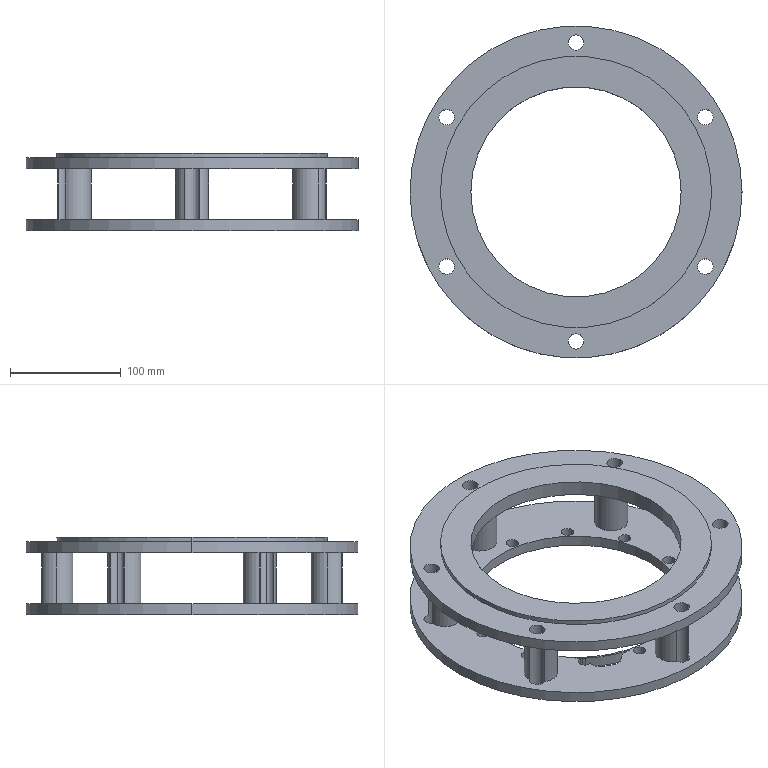Part | SolidWorks | features ICE 7, Extrusion 1 | 1 solid | 79 faces | box 300 x 300 x 69.96 mm | volume 1053348 mm3 | cylinder 74 | plane 5 | commonest cylinder face diameters 11 x25 30 x21 14 x12 190 x4 300 x4 20 x3